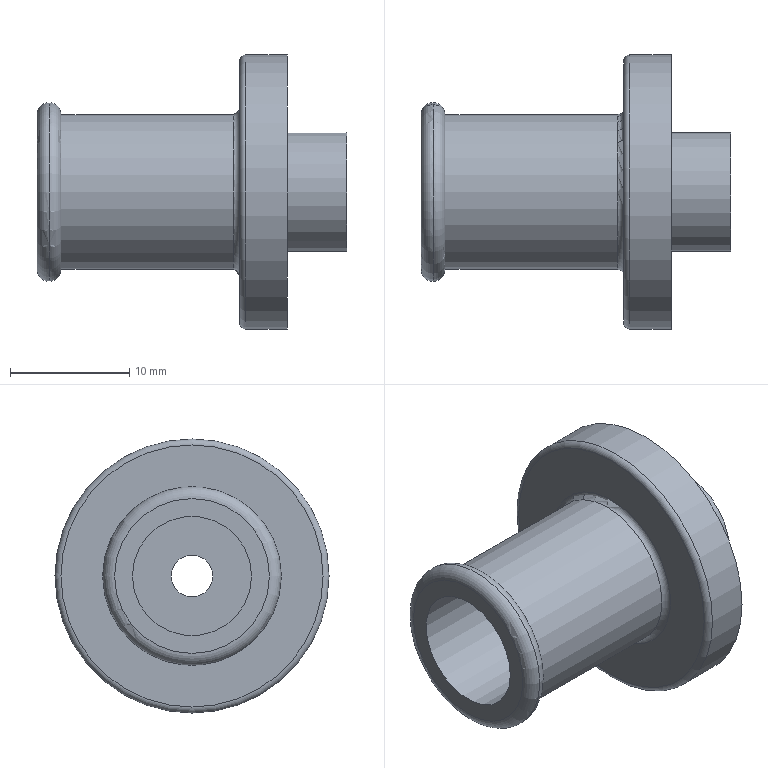Part | STEP file | 1-42.1 | 1 solid | 16 faces | box 26 x 23 x 23 mm | volume 2672 mm3 | cylinder 6 | plane 6 | torus 4 | commonest cylinder face diameters 10 x2 3.5 x1 8 x1 13 x1 23 x1
STEP:
#1=CARTESIAN_POINT('',(0.,0.,0.));
#2=DIRECTION('',(0.,0.,1.));
#3=DIRECTION('',(1.,0.,0.));
#4=AXIS2_PLACEMENT_3D('',#1,#2,#3);
#5=CARTESIAN_POINT('',(15.,5.,0.));
#6=VERTEX_POINT('',#5);
#7=CARTESIAN_POINT('',(15.,0.,0.));
#8=DIRECTION('',(-1.,0.,0.));
#9=DIRECTION('',(0.,1.,0.));
#10=AXIS2_PLACEMENT_3D('',#7,#8,#9);
#11=CIRCLE('',#10,5.);
#12=CARTESIAN_POINT('',(-2.,0.,0.));
#13=DIRECTION('',(1.,0.,0.));
#14=DIRECTION('',(0.,1.,0.));
#15=AXIS2_PLACEMENT_3D('',#12,#13,#14);
#16=CYLINDRICAL_SURFACE('',#15,5.);
#17=CARTESIAN_POINT('',(6.283,17.));
#18=DIRECTION('',(-1.,0.));
#19=VECTOR('',#18,1.);
#20=LINE('',#17,#19);
#21=(GEOMETRIC_REPRESENTATION_CONTEXT(2)PARAMETRIC_REPRESENTATION_CONTEXT()REPRESENTATION_CONTEXT('',''));
#22=DEFINITIONAL_REPRESENTATION('',(#20),#21);
#23=PCURVE('',#16,#22);
#24=CARTESIAN_POINT('',(15.,-5.75,0.));
#25=DIRECTION('',(1.,0.,0.));
#26=DIRECTION('',(0.,0.,-1.));
#27=AXIS2_PLACEMENT_3D('',#24,#25,#26);
#28=PLANE('',#27);
#29=CARTESIAN_POINT('',(0.,10.75));
#30=CARTESIAN_POINT('',(8.66,10.75));
#31=CARTESIAN_POINT('',(4.33,3.25));
#32=CARTESIAN_POINT('',(0.,-4.25));
#33=CARTESIAN_POINT('',(-4.33,3.25));
#34=CARTESIAN_POINT('',(-8.66,10.75));
#35=CARTESIAN_POINT('',(0.,10.75));
#36=(BOUNDED_CURVE()B_SPLINE_CURVE(2,(#29,#30,#31,#32,#33,#34,#35),.UNSPECIFIED.,.T.,.F.)B_SPLINE_CURVE_WITH_KNOTS((1,2,2,2,2,1),(-2.094,0.,2.094,4.189,6.283,8.378),.UNSPECIFIED.)CURVE()GEOMETRIC_REPRESENTATION_ITEM()RATIONAL_B_SPLINE_CURVE((1.,0.5,1.,0.5,1.,0.5,1.))REPRESENTATION_ITEM(''));
#37=(GEOMETRIC_REPRESENTATION_CONTEXT(2)PARAMETRIC_REPRESENTATION_CONTEXT()REPRESENTATION_CONTEXT('',''));
#38=DEFINITIONAL_REPRESENTATION('',(#36),#37);
#39=PCURVE('',#28,#38);
#40=SURFACE_CURVE('',#11,(#23,#39),.PCURVE_S1.);
#41=EDGE_CURVE('',#6,#6,#40,.T.);
#42=ORIENTED_EDGE('',*,*,#41,.T.);
#43=CARTESIAN_POINT('',(-2.,5.,0.));
#44=VERTEX_POINT('',#43);
#45=CARTESIAN_POINT('',(15.,5.,0.));
#46=DIRECTION('',(-1.,0.,0.));
#47=VECTOR('',#46,1.);
#48=LINE('',#45,#47);
#49=CARTESIAN_POINT('',(0.,17.));
#50=DIRECTION('',(0.,-1.));
#51=VECTOR('',#50,1.);
#52=LINE('',#49,#51);
#53=(GEOMETRIC_REPRESENTATION_CONTEXT(2)PARAMETRIC_REPRESENTATION_CONTEXT()REPRESENTATION_CONTEXT('',''));
#54=DEFINITIONAL_REPRESENTATION('',(#52),#53);
#55=PCURVE('',#16,#54);
#56=CARTESIAN_POINT('',(6.283,17.));
#57=DIRECTION('',(0.,-1.));
#58=VECTOR('',#57,1.);
#59=LINE('',#56,#58);
#60=(GEOMETRIC_REPRESENTATION_CONTEXT(2)PARAMETRIC_REPRESENTATION_CONTEXT()REPRESENTATION_CONTEXT('',''));
#61=DEFINITIONAL_REPRESENTATION('',(#59),#60);
#62=PCURVE('',#16,#61);
#63=SEAM_CURVE('',#48,(#55,#62),.PCURVE_S1.);
#64=EDGE_CURVE('',#6,#44,#63,.T.);
#65=ORIENTED_EDGE('',*,*,#64,.T.);
#66=CARTESIAN_POINT('',(-2.,0.,0.));
#67=DIRECTION('',(-1.,0.,0.));
#68=DIRECTION('',(0.,1.,0.));
#69=AXIS2_PLACEMENT_3D('',#66,#67,#68);
#70=CIRCLE('',#69,5.);
#71=CARTESIAN_POINT('',(6.283,0.));
#72=DIRECTION('',(-1.,0.));
#73=VECTOR('',#72,1.);
#74=LINE('',#71,#73);
#75=(GEOMETRIC_REPRESENTATION_CONTEXT(2)PARAMETRIC_REPRESENTATION_CONTEXT()REPRESENTATION_CONTEXT('',''));
#76=DEFINITIONAL_REPRESENTATION('',(#74),#75);
#77=PCURVE('',#16,#76);
#78=CARTESIAN_POINT('',(-2.,-2.01,0.));
#79=DIRECTION('',(1.,0.,0.));
#80=DIRECTION('',(0.,0.,-1.));
#81=AXIS2_PLACEMENT_3D('',#78,#79,#80);
#82=PLANE('',#81);
#83=CARTESIAN_POINT('',(0.,7.01));
#84=CARTESIAN_POINT('',(8.66,7.01));
#85=CARTESIAN_POINT('',(4.33,-0.4904));
#86=CARTESIAN_POINT('',(0.,-7.99));
#87=CARTESIAN_POINT('',(-4.33,-0.4904));
#88=CARTESIAN_POINT('',(-8.66,7.01));
#89=CARTESIAN_POINT('',(0.,7.01));
#90=(BOUNDED_CURVE()B_SPLINE_CURVE(2,(#83,#84,#85,#86,#87,#88,#89),.UNSPECIFIED.,.T.,.F.)B_SPLINE_CURVE_WITH_KNOTS((1,2,2,2,2,1),(-2.094,0.,2.094,4.189,6.283,8.378),.UNSPECIFIED.)CURVE()GEOMETRIC_REPRESENTATION_ITEM()RATIONAL_B_SPLINE_CURVE((1.,0.5,1.,0.5,1.,0.5,1.))REPRESENTATION_ITEM(''));
#91=(GEOMETRIC_REPRESENTATION_CONTEXT(2)PARAMETRIC_REPRESENTATION_CONTEXT()REPRESENTATION_CONTEXT('',''));
#92=DEFINITIONAL_REPRESENTATION('',(#90),#91);
#93=PCURVE('',#82,#92);
#94=SURFACE_CURVE('',#70,(#77,#93),.PCURVE_S1.);
#95=EDGE_CURVE('',#44,#44,#94,.T.);
#96=ORIENTED_EDGE('',*,*,#95,.F.);
#97=ORIENTED_EDGE('',*,*,#64,.F.);
#98=EDGE_LOOP('',(#42,#65,#96,#97));
#99=FACE_BOUND('',#98,.F.);
#100=ADVANCED_FACE('',(#99),#16,.F.);
#101=CARTESIAN_POINT('',(19.,11.5,0.));
#102=VERTEX_POINT('',#101);
#103=CARTESIAN_POINT('',(19.,0.,0.));
#104=DIRECTION('',(1.,0.,0.));
#105=DIRECTION('',(0.,1.,0.));
#106=AXIS2_PLACEMENT_3D('',#103,#104,#105);
#107=CIRCLE('',#106,11.5);
#108=CARTESIAN_POINT('',(19.,-3.081,0.));
#109=DIRECTION('',(1.,0.,0.));
#110=DIRECTION('',(0.,0.,-1.));
#111=AXIS2_PLACEMENT_3D('',#108,#109,#110);
#112=PLANE('',#111);
#113=CARTESIAN_POINT('',(0.,3.081));
#114=DIRECTION('',(0.,1.));
#115=AXIS2_PLACEMENT_2D('',#113,#114);
#116=CIRCLE('',#115,11.5);
#117=(GEOMETRIC_REPRESENTATION_CONTEXT(2)PARAMETRIC_REPRESENTATION_CONTEXT()REPRESENTATION_CONTEXT('',''));
#118=DEFINITIONAL_REPRESENTATION('',(#116),#117);
#119=PCURVE('',#112,#118);
#120=CARTESIAN_POINT('',(15.,0.,0.));
#121=DIRECTION('',(1.,0.,0.));
#122=DIRECTION('',(0.,1.,0.));
#123=AXIS2_PLACEMENT_3D('',#120,#121,#122);
#124=CYLINDRICAL_SURFACE('',#123,11.5);
#125=CARTESIAN_POINT('',(0.,4.));
#126=DIRECTION('',(1.,0.));
#127=VECTOR('',#126,1.);
#128=LINE('',#125,#127);
#129=(GEOMETRIC_REPRESENTATION_CONTEXT(2)PARAMETRIC_REPRESENTATION_CONTEXT()REPRESENTATION_CONTEXT('',''));
#130=DEFINITIONAL_REPRESENTATION('',(#128),#129);
#131=PCURVE('',#124,#130);
#132=SURFACE_CURVE('',#107,(#119,#131),.PCURVE_S1.);
#133=EDGE_CURVE('',#102,#102,#132,.T.);
#134=ORIENTED_EDGE('',*,*,#133,.T.);
#135=EDGE_LOOP('',(#134));
#136=FACE_BOUND('',#135,.T.);
#137=CARTESIAN_POINT('',(19.,5.,0.));
#138=VERTEX_POINT('',#137);
#139=CARTESIAN_POINT('',(19.,0.,0.));
#140=DIRECTION('',(1.,0.,0.));
#141=DIRECTION('',(0.,1.,0.));
#142=AXIS2_PLACEMENT_3D('',#139,#140,#141);
#143=CIRCLE('',#142,5.);
#144=CARTESIAN_POINT('',(0.,3.081));
#145=DIRECTION('',(0.,1.));
#146=AXIS2_PLACEMENT_2D('',#144,#145);
#147=CIRCLE('',#146,5.);
#148=(GEOMETRIC_REPRESENTATION_CONTEXT(2)PARAMETRIC_REPRESENTATION_CONTEXT()REPRESENTATION_CONTEXT('',''));
#149=DEFINITIONAL_REPRESENTATION('',(#147),#148);
#150=PCURVE('',#112,#149);
#151=CARTESIAN_POINT('',(19.,0.,0.));
#152=DIRECTION('',(1.,0.,0.));
#153=DIRECTION('',(0.,1.,0.));
#154=AXIS2_PLACEMENT_3D('',#151,#152,#153);
#155=CYLINDRICAL_SURFACE('',#154,5.);
#156=CARTESIAN_POINT('',(0.,0.));
#157=DIRECTION('',(1.,0.));
#158=VECTOR('',#157,1.);
#159=LINE('',#156,#158);
#160=(GEOMETRIC_REPRESENTATION_CONTEXT(2)PARAMETRIC_REPRESENTATION_CONTEXT()REPRESENTATION_CONTEXT('',''));
#161=DEFINITIONAL_REPRESENTATION('',(#159),#160);
#162=PCURVE('',#155,#161);
#163=SURFACE_CURVE('',#143,(#150,#162),.PCURVE_S1.);
#164=EDGE_CURVE('',#138,#138,#163,.T.);
#165=ORIENTED_EDGE('',*,*,#164,.F.);
#166=EDGE_LOOP('',(#165));
#167=FACE_BOUND('',#166,.T.);
#168=ADVANCED_FACE('',(#136,#167),#112,.T.);
#169=ORIENTED_EDGE('',*,*,#164,.T.);
#170=CARTESIAN_POINT('',(24.,5.,0.));
#171=VERTEX_POINT('',#170);
#172=CARTESIAN_POINT('',(19.,5.,0.));
#173=DIRECTION('',(1.,0.,0.));
#174=VECTOR('',#173,1.);
#175=LINE('',#172,#174);
#176=CARTESIAN_POINT('',(6.283,0.));
#177=DIRECTION('',(0.,1.));
#178=VECTOR('',#177,1.);
#179=LINE('',#176,#178);
#180=(GEOMETRIC_REPRESENTATION_CONTEXT(2)PARAMETRIC_REPRESENTATION_CONTEXT()REPRESENTATION_CONTEXT('',''));
#181=DEFINITIONAL_REPRESENTATION('',(#179),#180);
#182=PCURVE('',#155,#181);
#183=CARTESIAN_POINT('',(0.,0.));
#184=DIRECTION('',(0.,1.));
#185=VECTOR('',#184,1.);
#186=LINE('',#183,#185);
#187=(GEOMETRIC_REPRESENTATION_CONTEXT(2)PARAMETRIC_REPRESENTATION_CONTEXT()REPRESENTATION_CONTEXT('',''));
#188=DEFINITIONAL_REPRESENTATION('',(#186),#187);
#189=PCURVE('',#155,#188);
#190=SEAM_CURVE('',#175,(#182,#189),.PCURVE_S1.);
#191=EDGE_CURVE('',#138,#171,#190,.T.);
#192=ORIENTED_EDGE('',*,*,#191,.T.);
#193=CARTESIAN_POINT('',(24.,0.,0.));
#194=DIRECTION('',(1.,0.,0.));
#195=DIRECTION('',(0.,1.,0.));
#196=AXIS2_PLACEMENT_3D('',#193,#194,#195);
#197=CIRCLE('',#196,5.);
#198=CARTESIAN_POINT('',(0.,5.));
#199=DIRECTION('',(1.,0.));
#200=VECTOR('',#199,1.);
#201=LINE('',#198,#200);
#202=(GEOMETRIC_REPRESENTATION_CONTEXT(2)PARAMETRIC_REPRESENTATION_CONTEXT()REPRESENTATION_CONTEXT('',''));
#203=DEFINITIONAL_REPRESENTATION('',(#201),#202);
#204=PCURVE('',#155,#203);
#205=CARTESIAN_POINT('',(24.,-1.34,0.));
#206=DIRECTION('',(1.,0.,0.));
#207=DIRECTION('',(0.,0.,-1.));
#208=AXIS2_PLACEMENT_3D('',#205,#206,#207);
#209=PLANE('',#208);
#210=CARTESIAN_POINT('',(0.,1.34));
#211=DIRECTION('',(0.,1.));
#212=AXIS2_PLACEMENT_2D('',#210,#211);
#213=CIRCLE('',#212,5.);
#214=(GEOMETRIC_REPRESENTATION_CONTEXT(2)PARAMETRIC_REPRESENTATION_CONTEXT()REPRESENTATION_CONTEXT('',''));
#215=DEFINITIONAL_REPRESENTATION('',(#213),#214);
#216=PCURVE('',#209,#215);
#217=SURFACE_CURVE('',#197,(#204,#216),.PCURVE_S1.);
#218=EDGE_CURVE('',#171,#171,#217,.T.);
#219=ORIENTED_EDGE('',*,*,#218,.F.);
#220=ORIENTED_EDGE('',*,*,#191,.F.);
#221=EDGE_LOOP('',(#169,#192,#219,#220));
#222=FACE_BOUND('',#221,.T.);
#223=ADVANCED_FACE('',(#222),#155,.T.);
#224=ORIENTED_EDGE('',*,*,#41,.F.);
#225=EDGE_LOOP('',(#224));
#226=FACE_BOUND('',#225,.F.);
#227=CARTESIAN_POINT('',(15.,1.75,0.));
#228=VERTEX_POINT('',#227);
#229=CARTESIAN_POINT('',(15.,0.,0.));
#230=DIRECTION('',(1.,0.,0.));
#231=DIRECTION('',(0.,1.,0.));
#232=AXIS2_PLACEMENT_3D('',#229,#230,#231);
#233=CIRCLE('',#232,1.75);
#234=CARTESIAN_POINT('',(0.,5.75));
#235=DIRECTION('',(0.,1.));
#236=AXIS2_PLACEMENT_2D('',#234,#235);
#237=CIRCLE('',#236,1.75);
#238=(GEOMETRIC_REPRESENTATION_CONTEXT(2)PARAMETRIC_REPRESENTATION_CONTEXT()REPRESENTATION_CONTEXT('',''));
#239=DEFINITIONAL_REPRESENTATION('',(#237),#238);
#240=PCURVE('',#28,#239);
#241=CARTESIAN_POINT('',(15.,0.,0.));
#242=DIRECTION('',(1.,0.,0.));
#243=DIRECTION('',(0.,1.,0.));
#244=AXIS2_PLACEMENT_3D('',#241,#242,#243);
#245=CYLINDRICAL_SURFACE('',#244,1.75);
#246=CARTESIAN_POINT('',(0.,0.));
#247=DIRECTION('',(1.,0.));
#248=VECTOR('',#247,1.);
#249=LINE('',#246,#248);
#250=(GEOMETRIC_REPRESENTATION_CONTEXT(2)PARAMETRIC_REPRESENTATION_CONTEXT()REPRESENTATION_CONTEXT('',''));
#251=DEFINITIONAL_REPRESENTATION('',(#249),#250);
#252=PCURVE('',#245,#251);
#253=SURFACE_CURVE('',#233,(#240,#252),.PCURVE_S1.);
#254=EDGE_CURVE('',#228,#228,#253,.T.);
#255=ORIENTED_EDGE('',*,*,#254,.F.);
#256=EDGE_LOOP('',(#255));
#257=FACE_BOUND('',#256,.F.);
#258=ADVANCED_FACE('',(#226,#257),#28,.F.);
#259=CARTESIAN_POINT('',(-2.,6.5,0.));
#260=VERTEX_POINT('',#259);
#261=CARTESIAN_POINT('',(-2.,0.,0.));
#262=DIRECTION('',(1.,0.,0.));
#263=DIRECTION('',(0.,1.,0.));
#264=AXIS2_PLACEMENT_3D('',#261,#262,#263);
#265=CIRCLE('',#264,6.5);
#266=CARTESIAN_POINT('',(0.,2.01));
#267=DIRECTION('',(0.,1.));
#268=AXIS2_PLACEMENT_2D('',#266,#267);
#269=CIRCLE('',#268,6.5);
#270=(GEOMETRIC_REPRESENTATION_CONTEXT(2)PARAMETRIC_REPRESENTATION_CONTEXT()REPRESENTATION_CONTEXT('',''));
#271=DEFINITIONAL_REPRESENTATION('',(#269),#270);
#272=PCURVE('',#82,#271);
#273=CARTESIAN_POINT('',(-1.,0.,0.));
#274=DIRECTION('',(-1.,0.,0.));
#275=DIRECTION('',(0.,1.,0.));
#276=AXIS2_PLACEMENT_3D('',#273,#274,#275);
#277=TOROIDAL_SURFACE('',#276,6.5,1.);
#278=CARTESIAN_POINT('',(6.283,1.571));
#279=DIRECTION('',(-1.,0.));
#280=VECTOR('',#279,1.);
#281=LINE('',#278,#280);
#282=(GEOMETRIC_REPRESENTATION_CONTEXT(2)PARAMETRIC_REPRESENTATION_CONTEXT()REPRESENTATION_CONTEXT('',''));
#283=DEFINITIONAL_REPRESENTATION('',(#281),#282);
#284=PCURVE('',#277,#283);
#285=SURFACE_CURVE('',#265,(#272,#284),.PCURVE_S1.);
#286=EDGE_CURVE('',#260,#260,#285,.T.);
#287=ORIENTED_EDGE('',*,*,#286,.T.);
#288=EDGE_LOOP('',(#287));
#289=FACE_BOUND('',#288,.F.);
#290=ORIENTED_EDGE('',*,*,#95,.T.);
#291=EDGE_LOOP('',(#290));
#292=FACE_BOUND('',#291,.F.);
#293=ADVANCED_FACE('',(#289,#292),#82,.F.);
#294=CARTESIAN_POINT('',(0.,6.5,0.));
#295=VERTEX_POINT('',#294);
#296=CARTESIAN_POINT('',(0.,0.,0.));
#297=DIRECTION('',(1.,0.,0.));
#298=DIRECTION('',(0.,1.,0.));
#299=AXIS2_PLACEMENT_3D('',#296,#297,#298);
#300=CIRCLE('',#299,6.5);
#301=CARTESIAN_POINT('',(-1.,0.,0.));
#302=DIRECTION('',(-1.,0.,0.));
#303=DIRECTION('',(0.,1.,0.));
#304=AXIS2_PLACEMENT_3D('',#301,#302,#303);
#305=TOROIDAL_SURFACE('',#304,6.5,1.);
#306=CARTESIAN_POINT('',(6.283,4.712));
#307=DIRECTION('',(-1.,0.));
#308=VECTOR('',#307,1.);
#309=LINE('',#306,#308);
#310=(GEOMETRIC_REPRESENTATION_CONTEXT(2)PARAMETRIC_REPRESENTATION_CONTEXT()REPRESENTATION_CONTEXT('',''));
#311=DEFINITIONAL_REPRESENTATION('',(#309),#310);
#312=PCURVE('',#305,#311);
#313=CARTESIAN_POINT('',(0.,0.,0.));
#314=DIRECTION('',(1.,0.,0.));
#315=DIRECTION('',(0.,1.,0.));
#316=AXIS2_PLACEMENT_3D('',#313,#314,#315);
#317=CYLINDRICAL_SURFACE('',#316,6.5);
#318=CARTESIAN_POINT('',(0.,0.));
#319=DIRECTION('',(1.,0.));
#320=VECTOR('',#319,1.);
#321=LINE('',#318,#320);
#322=(GEOMETRIC_REPRESENTATION_CONTEXT(2)PARAMETRIC_REPRESENTATION_CONTEXT()REPRESENTATION_CONTEXT('',''));
#323=DEFINITIONAL_REPRESENTATION('',(#321),#322);
#324=PCURVE('',#317,#323);
#325=SURFACE_CURVE('',#300,(#312,#324),.PCURVE_S1.);
#326=EDGE_CURVE('',#295,#295,#325,.T.);
#327=ORIENTED_EDGE('',*,*,#326,.F.);
#328=CARTESIAN_POINT('',(-1.,7.5,0.));
#329=VERTEX_POINT('',#328);
#330=CARTESIAN_POINT('',(-1.,6.5,0.));
#331=DIRECTION('',(0.,0.,1.));
#332=DIRECTION('',(1.,0.,0.));
#333=AXIS2_PLACEMENT_3D('',#330,#331,#332);
#334=CIRCLE('',#333,1.);
#335=CARTESIAN_POINT('',(6.283,4.712));
#336=DIRECTION('',(0.,1.));
#337=VECTOR('',#336,1.);
#338=LINE('',#335,#337);
#339=(GEOMETRIC_REPRESENTATION_CONTEXT(2)PARAMETRIC_REPRESENTATION_CONTEXT()REPRESENTATION_CONTEXT('',''));
#340=DEFINITIONAL_REPRESENTATION('',(#338),#339);
#341=PCURVE('',#305,#340);
#342=CARTESIAN_POINT('',(0.,4.712));
#343=DIRECTION('',(0.,1.));
#344=VECTOR('',#343,1.);
#345=LINE('',#342,#344);
#346=(GEOMETRIC_REPRESENTATION_CONTEXT(2)PARAMETRIC_REPRESENTATION_CONTEXT()REPRESENTATION_CONTEXT('',''));
#347=DEFINITIONAL_REPRESENTATION('',(#345),#346);
#348=PCURVE('',#305,#347);
#349=SEAM_CURVE('',#334,(#341,#348),.PCURVE_S1.);
#350=EDGE_CURVE('',#295,#329,#349,.T.);
#351=ORIENTED_EDGE('',*,*,#350,.T.);
#352=CARTESIAN_POINT('',(-1.,0.,0.));
#353=DIRECTION('',(1.,0.,0.));
#354=DIRECTION('',(0.,1.,0.));
#355=AXIS2_PLACEMENT_3D('',#352,#353,#354);
#356=CIRCLE('',#355,7.5);
#357=CARTESIAN_POINT('',(6.283,6.283));
#358=DIRECTION('',(-1.,0.));
#359=VECTOR('',#358,1.);
#360=LINE('',#357,#359);
#361=(GEOMETRIC_REPRESENTATION_CONTEXT(2)PARAMETRIC_REPRESENTATION_CONTEXT()REPRESENTATION_CONTEXT('',''));
#362=DEFINITIONAL_REPRESENTATION('',(#360),#361);
#363=PCURVE('',#305,#362);
#364=CARTESIAN_POINT('',(6.283,0.));
#365=DIRECTION('',(-1.,0.));
#366=VECTOR('',#365,1.);
#367=LINE('',#364,#366);
#368=(GEOMETRIC_REPRESENTATION_CONTEXT(2)PARAMETRIC_REPRESENTATION_CONTEXT()REPRESENTATION_CONTEXT('',''));
#369=DEFINITIONAL_REPRESENTATION('',(#367),#368);
#370=PCURVE('',#277,#369);
#371=SURFACE_CURVE('',#356,(#363,#370),.PCURVE_S1.);
#372=EDGE_CURVE('',#329,#329,#371,.T.);
#373=ORIENTED_EDGE('',*,*,#372,.T.);
#374=ORIENTED_EDGE('',*,*,#350,.F.);
#375=EDGE_LOOP('',(#327,#351,#373,#374));
#376=FACE_BOUND('',#375,.T.);
#377=ADVANCED_FACE('',(#376),#305,.T.);
#378=CARTESIAN_POINT('',(-1.,6.5,0.));
#379=DIRECTION('',(0.,0.,-1.));
#380=DIRECTION('',(-1.,0.,0.));
#381=AXIS2_PLACEMENT_3D('',#378,#379,#380);
#382=CIRCLE('',#381,1.);
#383=CARTESIAN_POINT('',(0.,1.571));
#384=DIRECTION('',(0.,-1.));
#385=VECTOR('',#384,1.);
#386=LINE('',#383,#385);
#387=(GEOMETRIC_REPRESENTATION_CONTEXT(2)PARAMETRIC_REPRESENTATION_CONTEXT()REPRESENTATION_CONTEXT('',''));
#388=DEFINITIONAL_REPRESENTATION('',(#386),#387);
#389=PCURVE('',#277,#388);
#390=CARTESIAN_POINT('',(6.283,1.571));
#391=DIRECTION('',(0.,-1.));
#392=VECTOR('',#391,1.);
#393=LINE('',#390,#392);
#394=(GEOMETRIC_REPRESENTATION_CONTEXT(2)PARAMETRIC_REPRESENTATION_CONTEXT()REPRESENTATION_CONTEXT('',''));
#395=DEFINITIONAL_REPRESENTATION('',(#393),#394);
#396=PCURVE('',#277,#395);
#397=SEAM_CURVE('',#382,(#389,#396),.PCURVE_S1.);
#398=EDGE_CURVE('',#260,#329,#397,.T.);
#399=ORIENTED_EDGE('',*,*,#398,.T.);
#400=ORIENTED_EDGE('',*,*,#372,.F.);
#401=ORIENTED_EDGE('',*,*,#398,.F.);
#402=ORIENTED_EDGE('',*,*,#286,.T.);
#403=EDGE_LOOP('',(#399,#400,#401,#402));
#404=FACE_BOUND('',#403,.T.);
#405=ADVANCED_FACE('',(#404),#277,.T.);
#406=ORIENTED_EDGE('',*,*,#326,.T.);
#407=CARTESIAN_POINT('',(14.5,6.5,0.));
#408=VERTEX_POINT('',#407);
#409=CARTESIAN_POINT('',(0.,6.5,0.));
#410=DIRECTION('',(1.,0.,0.));
#411=VECTOR('',#410,1.);
#412=LINE('',#409,#411);
#413=CARTESIAN_POINT('',(6.283,0.));
#414=DIRECTION('',(0.,1.));
#415=VECTOR('',#414,1.);
#416=LINE('',#413,#415);
#417=(GEOMETRIC_REPRESENTATION_CONTEXT(2)PARAMETRIC_REPRESENTATION_CONTEXT()REPRESENTATION_CONTEXT('',''));
#418=DEFINITIONAL_REPRESENTATION('',(#416),#417);
#419=PCURVE('',#317,#418);
#420=CARTESIAN_POINT('',(0.,0.));
#421=DIRECTION('',(0.,1.));
#422=VECTOR('',#421,1.);
#423=LINE('',#420,#422);
#424=(GEOMETRIC_REPRESENTATION_CONTEXT(2)PARAMETRIC_REPRESENTATION_CONTEXT()REPRESENTATION_CONTEXT('',''));
#425=DEFINITIONAL_REPRESENTATION('',(#423),#424);
#426=PCURVE('',#317,#425);
#427=SEAM_CURVE('',#412,(#419,#426),.PCURVE_S1.);
#428=EDGE_CURVE('',#295,#408,#427,.T.);
#429=ORIENTED_EDGE('',*,*,#428,.T.);
#430=CARTESIAN_POINT('',(14.5,0.,0.));
#431=DIRECTION('',(-1.,0.,0.));
#432=DIRECTION('',(0.,1.,0.));
#433=AXIS2_PLACEMENT_3D('',#430,#431,#432);
#434=CIRCLE('',#433,6.5);
#435=CARTESIAN_POINT('',(6.283,14.5));
#436=DIRECTION('',(-1.,0.));
#437=VECTOR('',#436,1.);
#438=LINE('',#435,#437);
#439=(GEOMETRIC_REPRESENTATION_CONTEXT(2)PARAMETRIC_REPRESENTATION_CONTEXT()REPRESENTATION_CONTEXT('',''));
#440=DEFINITIONAL_REPRESENTATION('',(#438),#439);
#441=PCURVE('',#317,#440);
#442=CARTESIAN_POINT('',(14.5,0.,0.));
#443=DIRECTION('',(1.,0.,0.));
#444=DIRECTION('',(0.,1.,0.));
#445=AXIS2_PLACEMENT_3D('',#442,#443,#444);
#446=TOROIDAL_SURFACE('',#445,7.,0.5);
#447=CARTESIAN_POINT('',(6.283,3.142));
#448=DIRECTION('',(-1.,0.));
#449=VECTOR('',#448,1.);
#450=LINE('',#447,#449);
#451=(GEOMETRIC_REPRESENTATION_CONTEXT(2)PARAMETRIC_REPRESENTATION_CONTEXT()REPRESENTATION_CONTEXT('',''));
#452=DEFINITIONAL_REPRESENTATION('',(#450),#451);
#453=PCURVE('',#446,#452);
#454=SURFACE_CURVE('',#434,(#441,#453),.PCURVE_S1.);
#455=EDGE_CURVE('',#408,#408,#454,.T.);
#456=ORIENTED_EDGE('',*,*,#455,.T.);
#457=ORIENTED_EDGE('',*,*,#428,.F.);
#458=EDGE_LOOP('',(#406,#429,#456,#457));
#459=FACE_BOUND('',#458,.T.);
#460=ADVANCED_FACE('',(#459),#317,.T.);
#461=CARTESIAN_POINT('',(15.,11.,0.));
#462=VERTEX_POINT('',#461);
#463=CARTESIAN_POINT('',(15.,0.,0.));
#464=DIRECTION('',(-1.,0.,0.));
#465=DIRECTION('',(0.,1.,0.));
#466=AXIS2_PLACEMENT_3D('',#463,#464,#465);
#467=CIRCLE('',#466,11.);
#468=CARTESIAN_POINT('',(15.,-5.75,0.));
#469=DIRECTION('',(1.,0.,0.));
#470=DIRECTION('',(0.,0.,-1.));
#471=AXIS2_PLACEMENT_3D('',#468,#469,#470);
#472=PLANE('',#471);
#473=CARTESIAN_POINT('',(0.,16.75));
#474=CARTESIAN_POINT('',(19.053,16.75));
#475=CARTESIAN_POINT('',(9.526,0.25));
#476=CARTESIAN_POINT('',(0.,-16.25));
#477=CARTESIAN_POINT('',(-9.526,0.25));
#478=CARTESIAN_POINT('',(-19.053,16.75));
#479=CARTESIAN_POINT('',(0.,16.75));
#480=(BOUNDED_CURVE()B_SPLINE_CURVE(2,(#473,#474,#475,#476,#477,#478,#479),.UNSPECIFIED.,.T.,.F.)B_SPLINE_CURVE_WITH_KNOTS((1,2,2,2,2,1),(-2.094,0.,2.094,4.189,6.283,8.378),.UNSPECIFIED.)CURVE()GEOMETRIC_REPRESENTATION_ITEM()RATIONAL_B_SPLINE_CURVE((1.,0.5,1.,0.5,1.,0.5,1.))REPRESENTATION_ITEM(''));
#481=(GEOMETRIC_REPRESENTATION_CONTEXT(2)PARAMETRIC_REPRESENTATION_CONTEXT()REPRESENTATION_CONTEXT('',''));
#482=DEFINITIONAL_REPRESENTATION('',(#480),#481);
#483=PCURVE('',#472,#482);
#484=CARTESIAN_POINT('',(15.5,0.,0.));
#485=DIRECTION('',(1.,0.,0.));
#486=DIRECTION('',(0.,1.,0.));
#487=AXIS2_PLACEMENT_3D('',#484,#485,#486);
#488=TOROIDAL_SURFACE('',#487,11.,0.5);
#489=CARTESIAN_POINT('',(6.283,4.712));
#490=DIRECTION('',(-1.,0.));
#491=VECTOR('',#490,1.);
#492=LINE('',#489,#491);
#493=(GEOMETRIC_REPRESENTATION_CONTEXT(2)PARAMETRIC_REPRESENTATION_CONTEXT()REPRESENTATION_CONTEXT('',''));
#494=DEFINITIONAL_REPRESENTATION('',(#492),#493);
#495=PCURVE('',#488,#494);
#496=SURFACE_CURVE('',#467,(#483,#495),.PCURVE_S1.);
#497=EDGE_CURVE('',#462,#462,#496,.T.);
#498=ORIENTED_EDGE('',*,*,#497,.F.);
#499=EDGE_LOOP('',(#498));
#500=FACE_BOUND('',#499,.F.);
#501=CARTESIAN_POINT('',(15.,7.,0.));
#502=VERTEX_POINT('',#501);
#503=CARTESIAN_POINT('',(15.,0.,0.));
#504=DIRECTION('',(-1.,0.,0.));
#505=DIRECTION('',(0.,1.,0.));
#506=AXIS2_PLACEMENT_3D('',#503,#504,#505);
#507=CIRCLE('',#506,7.);
#508=CARTESIAN_POINT('',(0.,12.75));
#509=CARTESIAN_POINT('',(12.124,12.75));
#510=CARTESIAN_POINT('',(6.062,2.25));
#511=CARTESIAN_POINT('',(0.,-8.25));
#512=CARTESIAN_POINT('',(-6.062,2.25));
#513=CARTESIAN_POINT('',(-12.124,12.75));
#514=CARTESIAN_POINT('',(0.,12.75));
#515=(BOUNDED_CURVE()B_SPLINE_CURVE(2,(#508,#509,#510,#511,#512,#513,#514),.UNSPECIFIED.,.T.,.F.)B_SPLINE_CURVE_WITH_KNOTS((1,2,2,2,2,1),(-2.094,0.,2.094,4.189,6.283,8.378),.UNSPECIFIED.)CURVE()GEOMETRIC_REPRESENTATION_ITEM()RATIONAL_B_SPLINE_CURVE((1.,0.5,1.,0.5,1.,0.5,1.))REPRESENTATION_ITEM(''));
#516=(GEOMETRIC_REPRESENTATION_CONTEXT(2)PARAMETRIC_REPRESENTATION_CONTEXT()REPRESENTATION_CONTEXT('',''));
#517=DEFINITIONAL_REPRESENTATION('',(#515),#516);
#518=PCURVE('',#472,#517);
#519=CARTESIAN_POINT('',(6.283,1.571));
#520=DIRECTION('',(-1.,0.));
#521=VECTOR('',#520,1.);
#522=LINE('',#519,#521);
#523=(GEOMETRIC_REPRESENTATION_CONTEXT(2)PARAMETRIC_REPRESENTATION_CONTEXT()REPRESENTATION_CONTEXT('',''));
#524=DEFINITIONAL_REPRESENTATION('',(#522),#523);
#525=PCURVE('',#446,#524);
#526=SURFACE_CURVE('',#507,(#518,#525),.PCURVE_S1.);
#527=EDGE_CURVE('',#502,#502,#526,.T.);
#528=ORIENTED_EDGE('',*,*,#527,.T.);
#529=EDGE_LOOP('',(#528));
#530=FACE_BOUND('',#529,.F.);
#531=ADVANCED_FACE('',(#500,#530),#472,.F.);
#532=ORIENTED_EDGE('',*,*,#133,.F.);
#533=CARTESIAN_POINT('',(15.5,11.5,0.));
#534=VERTEX_POINT('',#533);
#535=CARTESIAN_POINT('',(15.5,11.5,0.));
#536=DIRECTION('',(1.,0.,0.));
#537=VECTOR('',#536,1.);
#538=LINE('',#535,#537);
#539=CARTESIAN_POINT('',(0.,0.5));
#540=DIRECTION('',(0.,1.));
#541=VECTOR('',#540,1.);
#542=LINE('',#539,#541);
#543=(GEOMETRIC_REPRESENTATION_CONTEXT(2)PARAMETRIC_REPRESENTATION_CONTEXT()REPRESENTATION_CONTEXT('',''));
#544=DEFINITIONAL_REPRESENTATION('',(#542),#543);
#545=PCURVE('',#124,#544);
#546=CARTESIAN_POINT('',(6.283,0.5));
#547=DIRECTION('',(0.,1.));
#548=VECTOR('',#547,1.);
#549=LINE('',#546,#548);
#550=(GEOMETRIC_REPRESENTATION_CONTEXT(2)PARAMETRIC_REPRESENTATION_CONTEXT()REPRESENTATION_CONTEXT('',''));
#551=DEFINITIONAL_REPRESENTATION('',(#549),#550);
#552=PCURVE('',#124,#551);
#553=SEAM_CURVE('',#538,(#545,#552),.PCURVE_S1.);
#554=EDGE_CURVE('',#534,#102,#553,.T.);
#555=ORIENTED_EDGE('',*,*,#554,.F.);
#556=CARTESIAN_POINT('',(15.5,0.,0.));
#557=DIRECTION('',(-1.,0.,0.));
#558=DIRECTION('',(0.,1.,0.));
#559=AXIS2_PLACEMENT_3D('',#556,#557,#558);
#560=CIRCLE('',#559,11.5);
#561=CARTESIAN_POINT('',(6.283,0.5));
#562=DIRECTION('',(-1.,0.));
#563=VECTOR('',#562,1.);
#564=LINE('',#561,#563);
#565=(GEOMETRIC_REPRESENTATION_CONTEXT(2)PARAMETRIC_REPRESENTATION_CONTEXT()REPRESENTATION_CONTEXT('',''));
#566=DEFINITIONAL_REPRESENTATION('',(#564),#565);
#567=PCURVE('',#124,#566);
#568=CARTESIAN_POINT('',(6.283,6.283));
#569=DIRECTION('',(-1.,0.));
#570=VECTOR('',#569,1.);
#571=LINE('',#568,#570);
#572=(GEOMETRIC_REPRESENTATION_CONTEXT(2)PARAMETRIC_REPRESENTATION_CONTEXT()REPRESENTATION_CONTEXT('',''));
#573=DEFINITIONAL_REPRESENTATION('',(#571),#572);
#574=PCURVE('',#488,#573);
#575=SURFACE_CURVE('',#560,(#567,#574),.PCURVE_S1.);
#576=EDGE_CURVE('',#534,#534,#575,.T.);
#577=ORIENTED_EDGE('',*,*,#576,.F.);
#578=ORIENTED_EDGE('',*,*,#554,.T.);
#579=EDGE_LOOP('',(#532,#555,#577,#578));
#580=FACE_BOUND('',#579,.T.);
#581=ADVANCED_FACE('',(#580),#124,.T.);
#582=ORIENTED_EDGE('',*,*,#527,.F.);
#583=CARTESIAN_POINT('',(14.5,7.,0.));
#584=DIRECTION('',(0.,0.,1.));
#585=DIRECTION('',(0.,-1.,0.));
#586=AXIS2_PLACEMENT_3D('',#583,#584,#585);
#587=CIRCLE('',#586,0.5);
#588=CARTESIAN_POINT('',(6.283,3.142));
#589=DIRECTION('',(0.,-1.));
#590=VECTOR('',#589,1.);
#591=LINE('',#588,#590);
#592=(GEOMETRIC_REPRESENTATION_CONTEXT(2)PARAMETRIC_REPRESENTATION_CONTEXT()REPRESENTATION_CONTEXT('',''));
#593=DEFINITIONAL_REPRESENTATION('',(#591),#592);
#594=PCURVE('',#446,#593);
#595=CARTESIAN_POINT('',(0.,3.142));
#596=DIRECTION('',(0.,-1.));
#597=VECTOR('',#596,1.);
#598=LINE('',#595,#597);
#599=(GEOMETRIC_REPRESENTATION_CONTEXT(2)PARAMETRIC_REPRESENTATION_CONTEXT()REPRESENTATION_CONTEXT('',''));
#600=DEFINITIONAL_REPRESENTATION('',(#598),#599);
#601=PCURVE('',#446,#600);
#602=SEAM_CURVE('',#587,(#594,#601),.PCURVE_S1.);
#603=EDGE_CURVE('',#408,#502,#602,.T.);
#604=ORIENTED_EDGE('',*,*,#603,.F.);
#605=ORIENTED_EDGE('',*,*,#455,.T.);
#606=ORIENTED_EDGE('',*,*,#603,.T.);
#607=EDGE_LOOP('',(#582,#604,#605,#606));
#608=FACE_BOUND('',#607,.F.);
#609=ADVANCED_FACE('',(#608),#446,.F.);
#610=ORIENTED_EDGE('',*,*,#497,.F.);
#611=CARTESIAN_POINT('',(15.5,11.,0.));
#612=DIRECTION('',(0.,0.,-1.));
#613=DIRECTION('',(-1.,0.,0.));
#614=AXIS2_PLACEMENT_3D('',#611,#612,#613);
#615=CIRCLE('',#614,0.5);
#616=CARTESIAN_POINT('',(6.283,4.712));
#617=DIRECTION('',(0.,1.));
#618=VECTOR('',#617,1.);
#619=LINE('',#616,#618);
#620=(GEOMETRIC_REPRESENTATION_CONTEXT(2)PARAMETRIC_REPRESENTATION_CONTEXT()REPRESENTATION_CONTEXT('',''));
#621=DEFINITIONAL_REPRESENTATION('',(#619),#620);
#622=PCURVE('',#488,#621);
#623=CARTESIAN_POINT('',(0.,4.712));
#624=DIRECTION('',(0.,1.));
#625=VECTOR('',#624,1.);
#626=LINE('',#623,#625);
#627=(GEOMETRIC_REPRESENTATION_CONTEXT(2)PARAMETRIC_REPRESENTATION_CONTEXT()REPRESENTATION_CONTEXT('',''));
#628=DEFINITIONAL_REPRESENTATION('',(#626),#627);
#629=PCURVE('',#488,#628);
#630=SEAM_CURVE('',#615,(#622,#629),.PCURVE_S1.);
#631=EDGE_CURVE('',#462,#534,#630,.T.);
#632=ORIENTED_EDGE('',*,*,#631,.T.);
#633=ORIENTED_EDGE('',*,*,#576,.T.);
#634=ORIENTED_EDGE('',*,*,#631,.F.);
#635=EDGE_LOOP('',(#610,#632,#633,#634));
#636=FACE_BOUND('',#635,.T.);
#637=ADVANCED_FACE('',(#636),#488,.T.);
#638=ORIENTED_EDGE('',*,*,#218,.T.);
#639=EDGE_LOOP('',(#638));
#640=FACE_BOUND('',#639,.T.);
#641=CARTESIAN_POINT('',(24.,4.,0.));
#642=VERTEX_POINT('',#641);
#643=CARTESIAN_POINT('',(24.,0.,0.));
#644=DIRECTION('',(1.,0.,0.));
#645=DIRECTION('',(0.,1.,0.));
#646=AXIS2_PLACEMENT_3D('',#643,#644,#645);
#647=CIRCLE('',#646,4.);
#648=CARTESIAN_POINT('',(0.,1.34));
#649=DIRECTION('',(0.,1.));
#650=AXIS2_PLACEMENT_2D('',#648,#649);
#651=CIRCLE('',#650,4.);
#652=(GEOMETRIC_REPRESENTATION_CONTEXT(2)PARAMETRIC_REPRESENTATION_CONTEXT()REPRESENTATION_CONTEXT('',''));
#653=DEFINITIONAL_REPRESENTATION('',(#651),#652);
#654=PCURVE('',#209,#653);
#655=CARTESIAN_POINT('',(24.,0.,0.));
#656=DIRECTION('',(-1.,0.,0.));
#657=DIRECTION('',(0.,1.,0.));
#658=AXIS2_PLACEMENT_3D('',#655,#656,#657);
#659=CYLINDRICAL_SURFACE('',#658,4.);
#660=CARTESIAN_POINT('',(6.283,0.));
#661=DIRECTION('',(-1.,0.));
#662=VECTOR('',#661,1.);
#663=LINE('',#660,#662);
#664=(GEOMETRIC_REPRESENTATION_CONTEXT(2)PARAMETRIC_REPRESENTATION_CONTEXT()REPRESENTATION_CONTEXT('',''));
#665=DEFINITIONAL_REPRESENTATION('',(#663),#664);
#666=PCURVE('',#659,#665);
#667=SURFACE_CURVE('',#647,(#654,#666),.PCURVE_S1.);
#668=EDGE_CURVE('',#642,#642,#667,.T.);
#669=ORIENTED_EDGE('',*,*,#668,.F.);
#670=EDGE_LOOP('',(#669));
#671=FACE_BOUND('',#670,.T.);
#672=ADVANCED_FACE('',(#640,#671),#209,.T.);
#673=ORIENTED_EDGE('',*,*,#254,.T.);
#674=CARTESIAN_POINT('',(17.,1.75,0.));
#675=VERTEX_POINT('',#674);
#676=CARTESIAN_POINT('',(15.,1.75,0.));
#677=DIRECTION('',(1.,0.,0.));
#678=VECTOR('',#677,1.);
#679=LINE('',#676,#678);
#680=CARTESIAN_POINT('',(6.283,0.));
#681=DIRECTION('',(0.,1.));
#682=VECTOR('',#681,1.);
#683=LINE('',#680,#682);
#684=(GEOMETRIC_REPRESENTATION_CONTEXT(2)PARAMETRIC_REPRESENTATION_CONTEXT()REPRESENTATION_CONTEXT('',''));
#685=DEFINITIONAL_REPRESENTATION('',(#683),#684);
#686=PCURVE('',#245,#685);
#687=CARTESIAN_POINT('',(0.,0.));
#688=DIRECTION('',(0.,1.));
#689=VECTOR('',#688,1.);
#690=LINE('',#687,#689);
#691=(GEOMETRIC_REPRESENTATION_CONTEXT(2)PARAMETRIC_REPRESENTATION_CONTEXT()REPRESENTATION_CONTEXT('',''));
#692=DEFINITIONAL_REPRESENTATION('',(#690),#691);
#693=PCURVE('',#245,#692);
#694=SEAM_CURVE('',#679,(#686,#693),.PCURVE_S1.);
#695=EDGE_CURVE('',#228,#675,#694,.T.);
#696=ORIENTED_EDGE('',*,*,#695,.T.);
#697=CARTESIAN_POINT('',(17.,0.,0.));
#698=DIRECTION('',(-1.,0.,0.));
#699=DIRECTION('',(0.,1.,0.));
#700=AXIS2_PLACEMENT_3D('',#697,#698,#699);
#701=CIRCLE('',#700,1.75);
#702=CARTESIAN_POINT('',(6.283,2.));
#703=DIRECTION('',(-1.,0.));
#704=VECTOR('',#703,1.);
#705=LINE('',#702,#704);
#706=(GEOMETRIC_REPRESENTATION_CONTEXT(2)PARAMETRIC_REPRESENTATION_CONTEXT()REPRESENTATION_CONTEXT('',''));
#707=DEFINITIONAL_REPRESENTATION('',(#705),#706);
#708=PCURVE('',#245,#707);
#709=CARTESIAN_POINT('',(17.,-1.072,0.));
#710=DIRECTION('',(1.,0.,0.));
#711=DIRECTION('',(0.,1.,0.));
#712=AXIS2_PLACEMENT_3D('',#709,#710,#711);
#713=PLANE('',#712);
#714=CARTESIAN_POINT('',(2.822,0.));
#715=CARTESIAN_POINT('',(2.822,-3.031));
#716=CARTESIAN_POINT('',(0.1968,-1.516));
#717=CARTESIAN_POINT('',(-2.428,0.));
#718=CARTESIAN_POINT('',(0.1968,1.516));
#719=CARTESIAN_POINT('',(2.822,3.031));
#720=CARTESIAN_POINT('',(2.822,0.));
#721=(BOUNDED_CURVE()B_SPLINE_CURVE(2,(#714,#715,#716,#717,#718,#719,#720),.UNSPECIFIED.,.T.,.F.)B_SPLINE_CURVE_WITH_KNOTS((1,2,2,2,2,1),(-2.094,0.,2.094,4.189,6.283,8.378),.UNSPECIFIED.)CURVE()GEOMETRIC_REPRESENTATION_ITEM()RATIONAL_B_SPLINE_CURVE((1.,0.5,1.,0.5,1.,0.5,1.))REPRESENTATION_ITEM(''));
#722=(GEOMETRIC_REPRESENTATION_CONTEXT(2)PARAMETRIC_REPRESENTATION_CONTEXT()REPRESENTATION_CONTEXT('',''));
#723=DEFINITIONAL_REPRESENTATION('',(#721),#722);
#724=PCURVE('',#713,#723);
#725=SURFACE_CURVE('',#701,(#708,#724),.PCURVE_S1.);
#726=EDGE_CURVE('',#675,#675,#725,.T.);
#727=ORIENTED_EDGE('',*,*,#726,.T.);
#728=ORIENTED_EDGE('',*,*,#695,.F.);
#729=EDGE_LOOP('',(#673,#696,#727,#728));
#730=FACE_BOUND('',#729,.F.);
#731=ADVANCED_FACE('',(#730),#245,.F.);
#732=CARTESIAN_POINT('',(17.,4.,0.));
#733=VERTEX_POINT('',#732);
#734=CARTESIAN_POINT('',(17.,0.,0.));
#735=DIRECTION('',(1.,0.,0.));
#736=DIRECTION('',(0.,1.,0.));
#737=AXIS2_PLACEMENT_3D('',#734,#735,#736);
#738=CIRCLE('',#737,4.);
#739=CARTESIAN_POINT('',(1.072,0.));
#740=DIRECTION('',(1.,0.));
#741=AXIS2_PLACEMENT_2D('',#739,#740);
#742=CIRCLE('',#741,4.);
#743=(GEOMETRIC_REPRESENTATION_CONTEXT(2)PARAMETRIC_REPRESENTATION_CONTEXT()REPRESENTATION_CONTEXT('',''));
#744=DEFINITIONAL_REPRESENTATION('',(#742),#743);
#745=PCURVE('',#713,#744);
#746=CARTESIAN_POINT('',(6.283,7.));
#747=DIRECTION('',(-1.,0.));
#748=VECTOR('',#747,1.);
#749=LINE('',#746,#748);
#750=(GEOMETRIC_REPRESENTATION_CONTEXT(2)PARAMETRIC_REPRESENTATION_CONTEXT()REPRESENTATION_CONTEXT('',''));
#751=DEFINITIONAL_REPRESENTATION('',(#749),#750);
#752=PCURVE('',#659,#751);
#753=SURFACE_CURVE('',#738,(#745,#752),.PCURVE_S1.);
#754=EDGE_CURVE('',#733,#733,#753,.T.);
#755=ORIENTED_EDGE('',*,*,#754,.T.);
#756=EDGE_LOOP('',(#755));
#757=FACE_BOUND('',#756,.T.);
#758=ORIENTED_EDGE('',*,*,#726,.T.);
#759=EDGE_LOOP('',(#758));
#760=FACE_BOUND('',#759,.T.);
#761=ADVANCED_FACE('',(#757,#760),#713,.T.);
#762=CARTESIAN_POINT('',(24.,4.,0.));
#763=DIRECTION('',(-1.,0.,0.));
#764=VECTOR('',#763,1.);
#765=LINE('',#762,#764);
#766=CARTESIAN_POINT('',(6.283,0.));
#767=DIRECTION('',(0.,1.));
#768=VECTOR('',#767,1.);
#769=LINE('',#766,#768);
#770=(GEOMETRIC_REPRESENTATION_CONTEXT(2)PARAMETRIC_REPRESENTATION_CONTEXT()REPRESENTATION_CONTEXT('',''));
#771=DEFINITIONAL_REPRESENTATION('',(#769),#770);
#772=PCURVE('',#659,#771);
#773=CARTESIAN_POINT('',(0.,0.));
#774=DIRECTION('',(0.,1.));
#775=VECTOR('',#774,1.);
#776=LINE('',#773,#775);
#777=(GEOMETRIC_REPRESENTATION_CONTEXT(2)PARAMETRIC_REPRESENTATION_CONTEXT()REPRESENTATION_CONTEXT('',''));
#778=DEFINITIONAL_REPRESENTATION('',(#776),#777);
#779=PCURVE('',#659,#778);
#780=SEAM_CURVE('',#765,(#772,#779),.PCURVE_S1.);
#781=EDGE_CURVE('',#642,#733,#780,.T.);
#782=ORIENTED_EDGE('',*,*,#781,.T.);
#783=ORIENTED_EDGE('',*,*,#754,.T.);
#784=ORIENTED_EDGE('',*,*,#781,.F.);
#785=ORIENTED_EDGE('',*,*,#668,.F.);
#786=EDGE_LOOP('',(#782,#783,#784,#785));
#787=FACE_BOUND('',#786,.F.);
#788=ADVANCED_FACE('',(#787),#659,.F.);
#789=CLOSED_SHELL('',(#100,#168,#223,#258,#293,#377,#405,#460,#531,#581,#609,#637,#672,#731,#761,#788));
#790=MANIFOLD_SOLID_BREP('',#789);
#791=(LENGTH_UNIT()NAMED_UNIT(*)SI_UNIT(.MILLI.,.METRE.));
#792=UNCERTAINTY_MEASURE_WITH_UNIT(LENGTH_MEASURE(0.0000001),#791,'','');
#793=(NAMED_UNIT(*)PLANE_ANGLE_UNIT()SI_UNIT($,.RADIAN.));
#794=(NAMED_UNIT(*)SI_UNIT($,.STERADIAN.)SOLID_ANGLE_UNIT());
#795=(GEOMETRIC_REPRESENTATION_CONTEXT(3)GLOBAL_UNCERTAINTY_ASSIGNED_CONTEXT((#792))GLOBAL_UNIT_ASSIGNED_CONTEXT((#791,#793,#794))REPRESENTATION_CONTEXT('',''));
#796=ADVANCED_BREP_SHAPE_REPRESENTATION('',(#4,#790),#795);